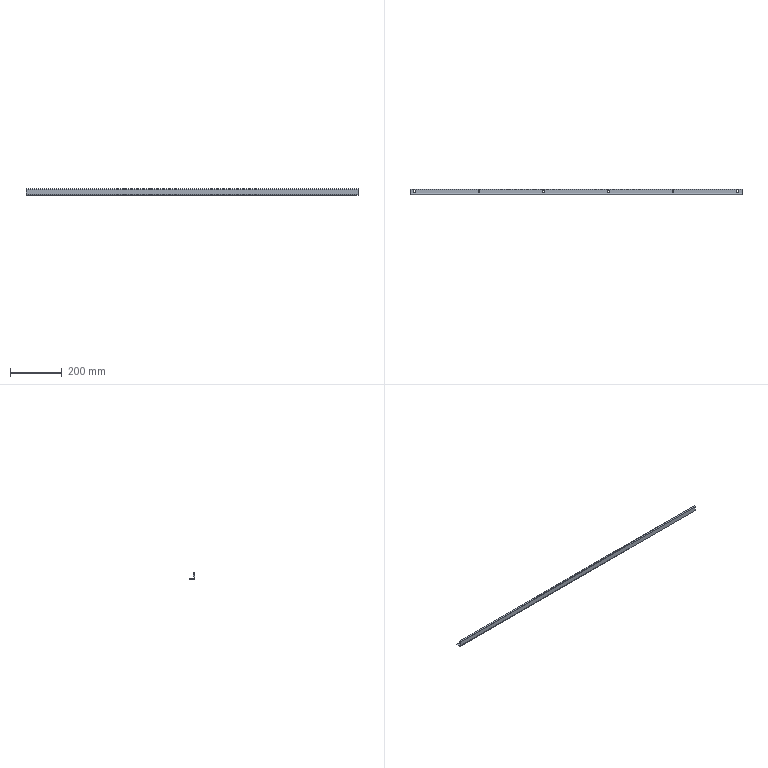Part | NX | features solid 2 | 1 solid | 68 faces | box 1284 x 20 x 25 mm | volume 140391 mm3 | plane 34 | cylinder 34 | commonest cylinder face diameters 6.5 x18 7 x12 2 x1 4 x1 6 x1 8 x1